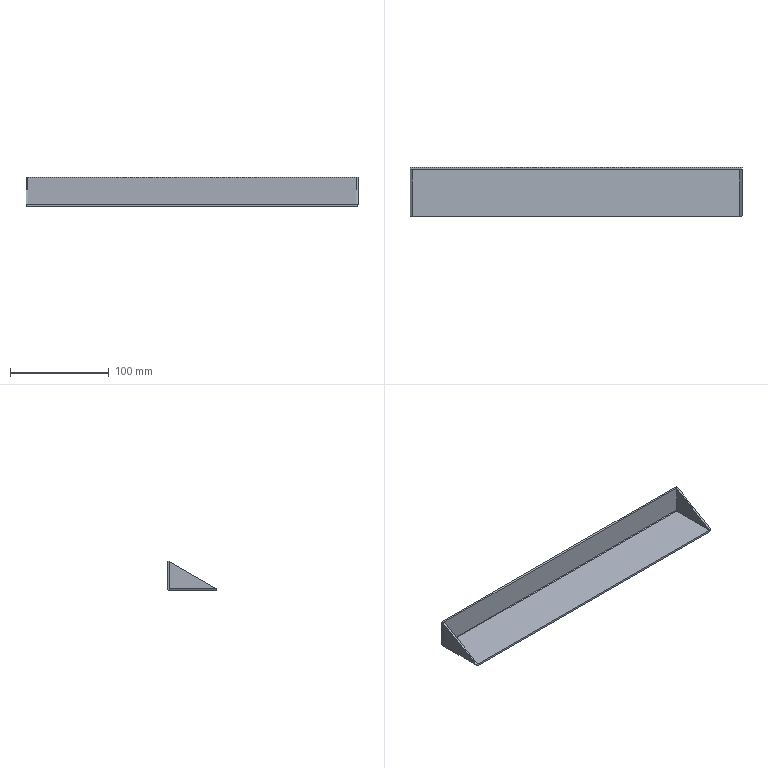Part | SolidWorks | features BaseBody 1 | 1 solid | 30 faces | box 336 x 50 x 30 mm | volume 54447 mm3 | plane 22 | cylinder 6 | spline 2 | commonest cylinder face diameters 1 x3 5 x3
STEP:
#1=CARTESIAN_POINT('',(166.,-24.136,0.5));
#2=VERTEX_POINT('',#1);
#3=CARTESIAN_POINT('',(166.,22.5,0.5));
#4=VERTEX_POINT('',#3);
#5=CARTESIAN_POINT('',(166.,-24.136,0.5));
#6=DIRECTION('',(0.,1.,0.));
#7=VECTOR('',#6,1000.);
#8=LINE('',#5,#7);
#9=EDGE_CURVE('',#2,#4,#8,.T.);
#10=ORIENTED_EDGE('',*,*,#9,.F.);
#11=CARTESIAN_POINT('',(166.,22.5,27.5));
#12=VERTEX_POINT('',#11);
#13=CARTESIAN_POINT('',(166.,22.5,27.5));
#14=DIRECTION('',(0.,-0.8654,-0.501));
#15=VECTOR('',#14,1000.);
#16=LINE('',#13,#15);
#17=EDGE_CURVE('',#12,#2,#16,.T.);
#18=ORIENTED_EDGE('',*,*,#17,.F.);
#19=CARTESIAN_POINT('',(166.,22.5,27.5));
#20=DIRECTION('',(0.,0.,1.));
#21=VECTOR('',#20,1000.);
#22=LINE('',#19,#21);
#23=EDGE_CURVE('',#4,#12,#22,.T.);
#24=ORIENTED_EDGE('',*,*,#23,.F.);
#25=EDGE_LOOP('',(#10,#18,#24));
#26=FACE_OUTER_BOUND('',#25,.T.);
#27=CARTESIAN_POINT('',(166.,0.,0.));
#28=DIRECTION('',(1.,0.,0.));
#29=DIRECTION('',(0.,0.,-1.));
#30=AXIS2_PLACEMENT_3D('',#27,#28,#29);
#31=PLANE('',#30);
#32=ADVANCED_FACE('',(#26),#31,.F.);
#33=CARTESIAN_POINT('',(168.,22.5,27.5));
#34=VERTEX_POINT('',#33);
#35=CARTESIAN_POINT('',(168.,-24.136,0.5));
#36=VERTEX_POINT('',#35);
#37=CARTESIAN_POINT('',(168.,-6.276,10.84));
#38=DIRECTION('',(0.,-0.8654,-0.501));
#39=VECTOR('',#38,1000.);
#40=LINE('',#37,#39);
#41=EDGE_CURVE('',#34,#36,#40,.T.);
#42=ORIENTED_EDGE('',*,*,#41,.T.);
#43=CARTESIAN_POINT('',(168.,22.5,0.5));
#44=VERTEX_POINT('',#43);
#45=CARTESIAN_POINT('',(168.,0.,0.5));
#46=DIRECTION('',(0.,1.,0.));
#47=VECTOR('',#46,1000.);
#48=LINE('',#45,#47);
#49=EDGE_CURVE('',#36,#44,#48,.T.);
#50=ORIENTED_EDGE('',*,*,#49,.T.);
#51=CARTESIAN_POINT('',(168.,22.5,0.));
#52=DIRECTION('',(0.,0.,1.));
#53=VECTOR('',#52,1000.);
#54=LINE('',#51,#53);
#55=EDGE_CURVE('',#44,#34,#54,.T.);
#56=ORIENTED_EDGE('',*,*,#55,.T.);
#57=EDGE_LOOP('',(#42,#50,#56));
#58=FACE_OUTER_BOUND('',#57,.T.);
#59=CARTESIAN_POINT('',(168.,0.,0.));
#60=DIRECTION('',(1.,0.,0.));
#61=DIRECTION('',(0.,0.,-1.));
#62=AXIS2_PLACEMENT_3D('',#59,#60,#61);
#63=PLANE('',#62);
#64=ADVANCED_FACE('',(#58),#63,.T.);
#65=CARTESIAN_POINT('',(166.,22.5,0.5));
#66=DIRECTION('',(1.,0.,0.));
#67=VECTOR('',#66,1000.);
#68=LINE('',#65,#67);
#69=EDGE_CURVE('',#4,#44,#68,.T.);
#70=ORIENTED_EDGE('',*,*,#69,.F.);
#71=ORIENTED_EDGE('',*,*,#23,.T.);
#72=CARTESIAN_POINT('',(168.,22.5,27.5));
#73=DIRECTION('',(-1.,0.,0.));
#74=VECTOR('',#73,1000.);
#75=LINE('',#72,#74);
#76=EDGE_CURVE('',#34,#12,#75,.T.);
#77=ORIENTED_EDGE('',*,*,#76,.F.);
#78=ORIENTED_EDGE('',*,*,#55,.F.);
#79=EDGE_LOOP('',(#70,#71,#77,#78));
#80=FACE_OUTER_BOUND('',#79,.T.);
#81=CARTESIAN_POINT('',(168.,22.5,27.5));
#82=DIRECTION('',(0.,-1.,0.));
#83=DIRECTION('',(-1.,0.,0.));
#84=AXIS2_PLACEMENT_3D('',#81,#82,#83);
#85=PLANE('',#84);
#86=ADVANCED_FACE('',(#80),#85,.F.);
#87=CARTESIAN_POINT('',(168.,-24.136,0.5));
#88=DIRECTION('',(1.,0.,0.));
#89=VECTOR('',#88,1000.);
#90=LINE('',#87,#89);
#91=EDGE_CURVE('',#2,#36,#90,.T.);
#92=ORIENTED_EDGE('',*,*,#91,.T.);
#93=ORIENTED_EDGE('',*,*,#41,.F.);
#94=ORIENTED_EDGE('',*,*,#76,.T.);
#95=ORIENTED_EDGE('',*,*,#17,.T.);
#96=EDGE_LOOP('',(#92,#93,#94,#95));
#97=FACE_OUTER_BOUND('',#96,.T.);
#98=CARTESIAN_POINT('',(168.,22.5,27.5));
#99=DIRECTION('',(0.,0.501,-0.8654));
#100=DIRECTION('',(-1.,0.,0.));
#101=AXIS2_PLACEMENT_3D('',#98,#99,#100);
#102=PLANE('',#101);
#103=ADVANCED_FACE('',(#97),#102,.F.);
#104=CARTESIAN_POINT('',(165.5,22.5,0.));
#105=VERTEX_POINT('',#104);
#106=CARTESIAN_POINT('',(165.5,-25.,0.));
#107=VERTEX_POINT('',#106);
#108=CARTESIAN_POINT('',(165.5,22.5,0.));
#109=DIRECTION('',(0.,-1.,0.));
#110=VECTOR('',#109,1000.);
#111=LINE('',#108,#110);
#112=EDGE_CURVE('',#105,#107,#111,.T.);
#113=ORIENTED_EDGE('',*,*,#112,.T.);
#114=CARTESIAN_POINT('',(165.5,-25.,0.));
#115=CARTESIAN_POINT('',(165.631,-24.856,0.));
#116=CARTESIAN_POINT('',(165.761,-24.712,0.05389));
#117=CARTESIAN_POINT('',(165.946,-24.424,0.239));
#118=CARTESIAN_POINT('',(166.,-24.28,0.3691));
#119=CARTESIAN_POINT('',(166.,-24.136,0.5));
#120=B_SPLINE_CURVE_WITH_KNOTS('',3,(#114,#115,#116,#117,#118,#119),.UNSPECIFIED.,.F.,.F.,(4,2,4),(0.,0.5,1.),.UNSPECIFIED.);
#121=EDGE_CURVE('',#107,#2,#120,.T.);
#122=ORIENTED_EDGE('',*,*,#121,.T.);
#123=ORIENTED_EDGE('',*,*,#9,.T.);
#124=CARTESIAN_POINT('',(165.5,22.5,0.5));
#125=DIRECTION('',(0.,1.,0.));
#126=DIRECTION('',(0.,0.,1.));
#127=AXIS2_PLACEMENT_3D('',#124,#125,#126);
#128=CIRCLE('',#127,0.5);
#129=EDGE_CURVE('',#4,#105,#128,.T.);
#130=ORIENTED_EDGE('',*,*,#129,.T.);
#131=EDGE_LOOP('',(#113,#122,#123,#130));
#132=FACE_OUTER_BOUND('',#131,.T.);
#133=CARTESIAN_POINT('',(165.5,22.5,0.5));
#134=DIRECTION('',(0.,1.,0.));
#135=DIRECTION('',(1.,0.,0.));
#136=AXIS2_PLACEMENT_3D('',#133,#134,#135);
#137=CYLINDRICAL_SURFACE('',#136,0.5);
#138=ADVANCED_FACE('',(#132),#137,.F.);
#139=CARTESIAN_POINT('',(165.5,22.5,-2.));
#140=VERTEX_POINT('',#139);
#141=CARTESIAN_POINT('',(165.5,-25.,-2.));
#142=VERTEX_POINT('',#141);
#143=CARTESIAN_POINT('',(165.5,22.5,-2.));
#144=DIRECTION('',(0.,-1.,0.));
#145=VECTOR('',#144,1000.);
#146=LINE('',#143,#145);
#147=EDGE_CURVE('',#140,#142,#146,.T.);
#148=ORIENTED_EDGE('',*,*,#147,.F.);
#149=CARTESIAN_POINT('',(165.5,22.5,0.5));
#150=DIRECTION('',(0.,1.,0.));
#151=DIRECTION('',(0.,0.,1.));
#152=AXIS2_PLACEMENT_3D('',#149,#150,#151);
#153=CIRCLE('',#152,2.5);
#154=EDGE_CURVE('',#44,#140,#153,.T.);
#155=ORIENTED_EDGE('',*,*,#154,.F.);
#156=ORIENTED_EDGE('',*,*,#49,.F.);
#157=CARTESIAN_POINT('',(165.5,-25.,-2.));
#158=CARTESIAN_POINT('',(165.827,-24.928,-2.));
#159=CARTESIAN_POINT('',(166.154,-24.856,-1.935));
#160=CARTESIAN_POINT('',(166.759,-24.712,-1.684));
#161=CARTESIAN_POINT('',(167.036,-24.64,-1.499));
#162=CARTESIAN_POINT('',(167.499,-24.496,-1.036));
#163=CARTESIAN_POINT('',(167.684,-24.424,-0.759));
#164=CARTESIAN_POINT('',(167.935,-24.28,-0.1544));
#165=CARTESIAN_POINT('',(168.,-24.208,0.1727));
#166=CARTESIAN_POINT('',(168.,-24.136,0.5));
#167=B_SPLINE_CURVE_WITH_KNOTS('',3,(#157,#158,#159,#160,#161,#162,#163,#164,#165,#166),.UNSPECIFIED.,.F.,.F.,(4,2,2,2,4),(0.,0.25,0.5,0.75,1.),.UNSPECIFIED.);
#168=EDGE_CURVE('',#142,#36,#167,.T.);
#169=ORIENTED_EDGE('',*,*,#168,.F.);
#170=EDGE_LOOP('',(#148,#155,#156,#169));
#171=FACE_OUTER_BOUND('',#170,.T.);
#172=CARTESIAN_POINT('',(165.5,22.5,0.5));
#173=DIRECTION('',(0.,1.,0.));
#174=DIRECTION('',(1.,0.,0.));
#175=AXIS2_PLACEMENT_3D('',#172,#173,#174);
#176=CYLINDRICAL_SURFACE('',#175,2.5);
#177=ADVANCED_FACE('',(#171),#176,.T.);
#178=ORIENTED_EDGE('',*,*,#129,.F.);
#179=ORIENTED_EDGE('',*,*,#69,.T.);
#180=ORIENTED_EDGE('',*,*,#154,.T.);
#181=CARTESIAN_POINT('',(165.5,22.5,0.));
#182=DIRECTION('',(0.,0.,-1.));
#183=VECTOR('',#182,1000.);
#184=LINE('',#181,#183);
#185=EDGE_CURVE('',#105,#140,#184,.T.);
#186=ORIENTED_EDGE('',*,*,#185,.F.);
#187=EDGE_LOOP('',(#178,#179,#180,#186));
#188=FACE_OUTER_BOUND('',#187,.T.);
#189=CARTESIAN_POINT('',(165.5,22.5,0.5));
#190=DIRECTION('',(0.,-1.,0.));
#191=DIRECTION('',(0.,0.,-1.));
#192=AXIS2_PLACEMENT_3D('',#189,#190,#191);
#193=PLANE('',#192);
#194=ADVANCED_FACE('',(#188),#193,.F.);
#195=ORIENTED_EDGE('',*,*,#91,.F.);
#196=ORIENTED_EDGE('',*,*,#121,.F.);
#197=CARTESIAN_POINT('',(165.5,-25.,0.));
#198=DIRECTION('',(0.,0.,-1.));
#199=VECTOR('',#198,1000.);
#200=LINE('',#197,#199);
#201=EDGE_CURVE('',#107,#142,#200,.T.);
#202=ORIENTED_EDGE('',*,*,#201,.T.);
#203=ORIENTED_EDGE('',*,*,#168,.T.);
#204=EDGE_LOOP('',(#195,#196,#202,#203));
#205=FACE_OUTER_BOUND('',#204,.T.);
#206=CARTESIAN_POINT('',(165.5,-25.,-2.02));
#207=CARTESIAN_POINT('',(165.83,-24.928,-2.02));
#208=CARTESIAN_POINT('',(166.16,-24.856,-1.954));
#209=CARTESIAN_POINT('',(166.769,-24.712,-1.702));
#210=CARTESIAN_POINT('',(167.049,-24.64,-1.515));
#211=CARTESIAN_POINT('',(167.515,-24.496,-1.049));
#212=CARTESIAN_POINT('',(167.702,-24.424,-0.7691));
#213=CARTESIAN_POINT('',(167.954,-24.28,-0.1596));
#214=CARTESIAN_POINT('',(168.02,-24.208,0.1701));
#215=CARTESIAN_POINT('',(168.02,-24.136,0.5));
#216=CARTESIAN_POINT('',(165.5,-25.,-2.));
#217=CARTESIAN_POINT('',(165.827,-24.928,-2.));
#218=CARTESIAN_POINT('',(166.154,-24.856,-1.935));
#219=CARTESIAN_POINT('',(166.759,-24.712,-1.684));
#220=CARTESIAN_POINT('',(167.036,-24.64,-1.499));
#221=CARTESIAN_POINT('',(167.499,-24.496,-1.036));
#222=CARTESIAN_POINT('',(167.684,-24.424,-0.759));
#223=CARTESIAN_POINT('',(167.935,-24.28,-0.1544));
#224=CARTESIAN_POINT('',(168.,-24.208,0.1727));
#225=CARTESIAN_POINT('',(168.,-24.136,0.5));
#226=CARTESIAN_POINT('',(165.5,-25.,0.));
#227=CARTESIAN_POINT('',(165.565,-24.928,0.));
#228=CARTESIAN_POINT('',(165.631,-24.856,0.01301));
#229=CARTESIAN_POINT('',(165.752,-24.712,0.06311));
#230=CARTESIAN_POINT('',(165.807,-24.64,0.1002));
#231=CARTESIAN_POINT('',(165.9,-24.496,0.1927));
#232=CARTESIAN_POINT('',(165.937,-24.424,0.2482));
#233=CARTESIAN_POINT('',(165.987,-24.28,0.3691));
#234=CARTESIAN_POINT('',(166.,-24.208,0.4345));
#235=CARTESIAN_POINT('',(166.,-24.136,0.5));
#236=CARTESIAN_POINT('',(165.5,-25.,0.0202));
#237=CARTESIAN_POINT('',(165.563,-24.928,0.0202));
#238=CARTESIAN_POINT('',(165.626,-24.856,0.03269));
#239=CARTESIAN_POINT('',(165.742,-24.712,0.08076));
#240=CARTESIAN_POINT('',(165.795,-24.64,0.1163));
#241=CARTESIAN_POINT('',(165.884,-24.496,0.2051));
#242=CARTESIAN_POINT('',(165.919,-24.424,0.2584));
#243=CARTESIAN_POINT('',(165.967,-24.28,0.3744));
#244=CARTESIAN_POINT('',(165.98,-24.208,0.4372));
#245=CARTESIAN_POINT('',(165.98,-24.136,0.5));
#246=B_SPLINE_SURFACE_WITH_KNOTS('',1,3,((#206,#207,#208,#209,#210,#211,#212,#213,#214,#215),(#216,#217,#218,#219,#220,#221,#222,#223,#224,#225),(#226,#227,#228,#229,#230,#231,#232,#233,#234,#235),(#236,#237,#238,#239,#240,#241,#242,#243,#244,#245)),.UNSPECIFIED.,.F.,.F.,.F.,(2,1,1,2),(4,2,2,2,4),(-0.01,0.,1.,1.01),(0.,0.25,0.5,0.75,1.),.UNSPECIFIED.);
#247=ADVANCED_FACE('',(#205),#246,.F.);
#248=CARTESIAN_POINT('',(-166.,-24.136,0.5));
#249=VERTEX_POINT('',#248);
#250=CARTESIAN_POINT('',(-166.,22.5,27.5));
#251=VERTEX_POINT('',#250);
#252=CARTESIAN_POINT('',(-166.,22.5,27.5));
#253=DIRECTION('',(0.,0.8654,0.501));
#254=VECTOR('',#253,1000.);
#255=LINE('',#252,#254);
#256=EDGE_CURVE('',#249,#251,#255,.T.);
#257=ORIENTED_EDGE('',*,*,#256,.F.);
#258=CARTESIAN_POINT('',(-166.,22.5,0.5));
#259=VERTEX_POINT('',#258);
#260=CARTESIAN_POINT('',(-166.,22.5,0.5));
#261=DIRECTION('',(0.,-1.,0.));
#262=VECTOR('',#261,1000.);
#263=LINE('',#260,#262);
#264=EDGE_CURVE('',#259,#249,#263,.T.);
#265=ORIENTED_EDGE('',*,*,#264,.F.);
#266=CARTESIAN_POINT('',(-166.,22.5,0.));
#267=DIRECTION('',(0.,0.,-1.));
#268=VECTOR('',#267,1000.);
#269=LINE('',#266,#268);
#270=EDGE_CURVE('',#251,#259,#269,.T.);
#271=ORIENTED_EDGE('',*,*,#270,.F.);
#272=EDGE_LOOP('',(#257,#265,#271));
#273=FACE_OUTER_BOUND('',#272,.T.);
#274=CARTESIAN_POINT('',(-166.,0.,0.));
#275=DIRECTION('',(1.,0.,0.));
#276=DIRECTION('',(0.,0.,1.));
#277=AXIS2_PLACEMENT_3D('',#274,#275,#276);
#278=PLANE('',#277);
#279=ADVANCED_FACE('',(#273),#278,.T.);
#280=CARTESIAN_POINT('',(-168.,-24.136,0.5));
#281=VERTEX_POINT('',#280);
#282=CARTESIAN_POINT('',(-168.,22.5,0.5));
#283=VERTEX_POINT('',#282);
#284=CARTESIAN_POINT('',(-168.,22.5,0.5));
#285=DIRECTION('',(0.,1.,0.));
#286=VECTOR('',#285,1000.);
#287=LINE('',#284,#286);
#288=EDGE_CURVE('',#281,#283,#287,.T.);
#289=ORIENTED_EDGE('',*,*,#288,.F.);
#290=CARTESIAN_POINT('',(-168.,22.5,27.5));
#291=VERTEX_POINT('',#290);
#292=CARTESIAN_POINT('',(-168.,-6.276,10.84));
#293=DIRECTION('',(0.,0.8654,0.501));
#294=VECTOR('',#293,1000.);
#295=LINE('',#292,#294);
#296=EDGE_CURVE('',#281,#291,#295,.T.);
#297=ORIENTED_EDGE('',*,*,#296,.T.);
#298=CARTESIAN_POINT('',(-168.,22.5,0.));
#299=DIRECTION('',(0.,0.,-1.));
#300=VECTOR('',#299,1000.);
#301=LINE('',#298,#300);
#302=EDGE_CURVE('',#291,#283,#301,.T.);
#303=ORIENTED_EDGE('',*,*,#302,.T.);
#304=EDGE_LOOP('',(#289,#297,#303));
#305=FACE_OUTER_BOUND('',#304,.T.);
#306=CARTESIAN_POINT('',(-168.,0.,0.));
#307=DIRECTION('',(1.,0.,0.));
#308=DIRECTION('',(0.,0.,1.));
#309=AXIS2_PLACEMENT_3D('',#306,#307,#308);
#310=PLANE('',#309);
#311=ADVANCED_FACE('',(#305),#310,.F.);
#312=CARTESIAN_POINT('',(-166.,-24.136,0.5));
#313=DIRECTION('',(-1.,0.,0.));
#314=VECTOR('',#313,1000.);
#315=LINE('',#312,#314);
#316=EDGE_CURVE('',#249,#281,#315,.T.);
#317=ORIENTED_EDGE('',*,*,#316,.F.);
#318=ORIENTED_EDGE('',*,*,#256,.T.);
#319=CARTESIAN_POINT('',(-168.,22.5,27.5));
#320=DIRECTION('',(1.,0.,0.));
#321=VECTOR('',#320,1000.);
#322=LINE('',#319,#321);
#323=EDGE_CURVE('',#291,#251,#322,.T.);
#324=ORIENTED_EDGE('',*,*,#323,.F.);
#325=ORIENTED_EDGE('',*,*,#296,.F.);
#326=EDGE_LOOP('',(#317,#318,#324,#325));
#327=FACE_OUTER_BOUND('',#326,.T.);
#328=CARTESIAN_POINT('',(-168.,22.5,27.5));
#329=DIRECTION('',(0.,0.501,-0.8654));
#330=DIRECTION('',(-1.,0.,0.));
#331=AXIS2_PLACEMENT_3D('',#328,#329,#330);
#332=PLANE('',#331);
#333=ADVANCED_FACE('',(#327),#332,.F.);
#334=CARTESIAN_POINT('',(-168.,22.5,0.5));
#335=DIRECTION('',(-1.,0.,0.));
#336=VECTOR('',#335,1000.);
#337=LINE('',#334,#336);
#338=EDGE_CURVE('',#259,#283,#337,.T.);
#339=ORIENTED_EDGE('',*,*,#338,.T.);
#340=ORIENTED_EDGE('',*,*,#302,.F.);
#341=ORIENTED_EDGE('',*,*,#323,.T.);
#342=ORIENTED_EDGE('',*,*,#270,.T.);
#343=EDGE_LOOP('',(#339,#340,#341,#342));
#344=FACE_OUTER_BOUND('',#343,.T.);
#345=CARTESIAN_POINT('',(-168.,22.5,0.));
#346=DIRECTION('',(0.,-1.,0.));
#347=DIRECTION('',(-1.,0.,0.));
#348=AXIS2_PLACEMENT_3D('',#345,#346,#347);
#349=PLANE('',#348);
#350=ADVANCED_FACE('',(#344),#349,.F.);
#351=CARTESIAN_POINT('',(-165.5,-25.,0.));
#352=VERTEX_POINT('',#351);
#353=CARTESIAN_POINT('',(-165.5,22.5,0.));
#354=VERTEX_POINT('',#353);
#355=CARTESIAN_POINT('',(-165.5,-25.,0.));
#356=DIRECTION('',(0.,1.,0.));
#357=VECTOR('',#356,1000.);
#358=LINE('',#355,#357);
#359=EDGE_CURVE('',#352,#354,#358,.T.);
#360=ORIENTED_EDGE('',*,*,#359,.T.);
#361=CARTESIAN_POINT('',(-165.5,22.5,0.5));
#362=DIRECTION('',(0.,1.,0.));
#363=DIRECTION('',(0.,0.,-1.));
#364=AXIS2_PLACEMENT_3D('',#361,#362,#363);
#365=CIRCLE('',#364,0.5);
#366=EDGE_CURVE('',#354,#259,#365,.T.);
#367=ORIENTED_EDGE('',*,*,#366,.T.);
#368=ORIENTED_EDGE('',*,*,#264,.T.);
#369=CARTESIAN_POINT('',(-166.,-24.136,0.5));
#370=CARTESIAN_POINT('',(-166.,-24.28,0.3691));
#371=CARTESIAN_POINT('',(-165.946,-24.424,0.239));
#372=CARTESIAN_POINT('',(-165.761,-24.712,0.05389));
#373=CARTESIAN_POINT('',(-165.631,-24.856,0.));
#374=CARTESIAN_POINT('',(-165.5,-25.,0.));
#375=B_SPLINE_CURVE_WITH_KNOTS('',3,(#369,#370,#371,#372,#373,#374),.UNSPECIFIED.,.F.,.F.,(4,2,4),(0.,0.5,1.),.UNSPECIFIED.);
#376=EDGE_CURVE('',#249,#352,#375,.T.);
#377=ORIENTED_EDGE('',*,*,#376,.T.);
#378=EDGE_LOOP('',(#360,#367,#368,#377));
#379=FACE_OUTER_BOUND('',#378,.T.);
#380=CARTESIAN_POINT('',(-165.5,-25.,0.5));
#381=DIRECTION('',(0.,-1.,0.));
#382=DIRECTION('',(-1.,0.,0.));
#383=AXIS2_PLACEMENT_3D('',#380,#381,#382);
#384=CYLINDRICAL_SURFACE('',#383,0.5);
#385=ADVANCED_FACE('',(#379),#384,.F.);
#386=CARTESIAN_POINT('',(-165.5,-25.,-2.));
#387=VERTEX_POINT('',#386);
#388=CARTESIAN_POINT('',(-165.5,22.5,-2.));
#389=VERTEX_POINT('',#388);
#390=CARTESIAN_POINT('',(-165.5,-25.,-2.));
#391=DIRECTION('',(0.,1.,0.));
#392=VECTOR('',#391,1000.);
#393=LINE('',#390,#392);
#394=EDGE_CURVE('',#387,#389,#393,.T.);
#395=ORIENTED_EDGE('',*,*,#394,.F.);
#396=CARTESIAN_POINT('',(-168.,-24.136,0.5));
#397=CARTESIAN_POINT('',(-168.,-24.208,0.1727));
#398=CARTESIAN_POINT('',(-167.935,-24.28,-0.1544));
#399=CARTESIAN_POINT('',(-167.684,-24.424,-0.759));
#400=CARTESIAN_POINT('',(-167.499,-24.496,-1.036));
#401=CARTESIAN_POINT('',(-167.036,-24.64,-1.499));
#402=CARTESIAN_POINT('',(-166.759,-24.712,-1.684));
#403=CARTESIAN_POINT('',(-166.154,-24.856,-1.935));
#404=CARTESIAN_POINT('',(-165.827,-24.928,-2.));
#405=CARTESIAN_POINT('',(-165.5,-25.,-2.));
#406=B_SPLINE_CURVE_WITH_KNOTS('',3,(#396,#397,#398,#399,#400,#401,#402,#403,#404,#405),.UNSPECIFIED.,.F.,.F.,(4,2,2,2,4),(0.,0.25,0.5,0.75,1.),.UNSPECIFIED.);
#407=EDGE_CURVE('',#281,#387,#406,.T.);
#408=ORIENTED_EDGE('',*,*,#407,.F.);
#409=ORIENTED_EDGE('',*,*,#288,.T.);
#410=CARTESIAN_POINT('',(-165.5,22.5,0.5));
#411=DIRECTION('',(0.,1.,0.));
#412=DIRECTION('',(0.,0.,-1.));
#413=AXIS2_PLACEMENT_3D('',#410,#411,#412);
#414=CIRCLE('',#413,2.5);
#415=EDGE_CURVE('',#389,#283,#414,.T.);
#416=ORIENTED_EDGE('',*,*,#415,.F.);
#417=EDGE_LOOP('',(#395,#408,#409,#416));
#418=FACE_OUTER_BOUND('',#417,.T.);
#419=CARTESIAN_POINT('',(-165.5,-25.,0.5));
#420=DIRECTION('',(0.,-1.,0.));
#421=DIRECTION('',(-1.,0.,0.));
#422=AXIS2_PLACEMENT_3D('',#419,#420,#421);
#423=CYLINDRICAL_SURFACE('',#422,2.5);
#424=ADVANCED_FACE('',(#418),#423,.T.);
#425=ORIENTED_EDGE('',*,*,#376,.F.);
#426=ORIENTED_EDGE('',*,*,#316,.T.);
#427=ORIENTED_EDGE('',*,*,#407,.T.);
#428=CARTESIAN_POINT('',(-165.5,-25.,0.));
#429=DIRECTION('',(0.,0.,-1.));
#430=VECTOR('',#429,1000.);
#431=LINE('',#428,#430);
#432=EDGE_CURVE('',#352,#387,#431,.T.);
#433=ORIENTED_EDGE('',*,*,#432,.F.);
#434=EDGE_LOOP('',(#425,#426,#427,#433));
#435=FACE_OUTER_BOUND('',#434,.T.);
#436=CARTESIAN_POINT('',(-168.02,-24.136,0.5));
#437=CARTESIAN_POINT('',(-168.02,-24.208,0.1701));
#438=CARTESIAN_POINT('',(-167.954,-24.28,-0.1596));
#439=CARTESIAN_POINT('',(-167.702,-24.424,-0.7691));
#440=CARTESIAN_POINT('',(-167.515,-24.496,-1.049));
#441=CARTESIAN_POINT('',(-167.049,-24.64,-1.515));
#442=CARTESIAN_POINT('',(-166.769,-24.712,-1.702));
#443=CARTESIAN_POINT('',(-166.16,-24.856,-1.954));
#444=CARTESIAN_POINT('',(-165.83,-24.928,-2.02));
#445=CARTESIAN_POINT('',(-165.5,-25.,-2.02));
#446=CARTESIAN_POINT('',(-168.,-24.136,0.5));
#447=CARTESIAN_POINT('',(-168.,-24.208,0.1727));
#448=CARTESIAN_POINT('',(-167.935,-24.28,-0.1544));
#449=CARTESIAN_POINT('',(-167.684,-24.424,-0.759));
#450=CARTESIAN_POINT('',(-167.499,-24.496,-1.036));
#451=CARTESIAN_POINT('',(-167.036,-24.64,-1.499));
#452=CARTESIAN_POINT('',(-166.759,-24.712,-1.684));
#453=CARTESIAN_POINT('',(-166.154,-24.856,-1.935));
#454=CARTESIAN_POINT('',(-165.827,-24.928,-2.));
#455=CARTESIAN_POINT('',(-165.5,-25.,-2.));
#456=CARTESIAN_POINT('',(-166.,-24.136,0.5));
#457=CARTESIAN_POINT('',(-166.,-24.208,0.4345));
#458=CARTESIAN_POINT('',(-165.987,-24.28,0.3691));
#459=CARTESIAN_POINT('',(-165.937,-24.424,0.2482));
#460=CARTESIAN_POINT('',(-165.9,-24.496,0.1927));
#461=CARTESIAN_POINT('',(-165.807,-24.64,0.1002));
#462=CARTESIAN_POINT('',(-165.752,-24.712,0.06311));
#463=CARTESIAN_POINT('',(-165.631,-24.856,0.01301));
#464=CARTESIAN_POINT('',(-165.565,-24.928,0.));
#465=CARTESIAN_POINT('',(-165.5,-25.,0.));
#466=CARTESIAN_POINT('',(-165.98,-24.136,0.5));
#467=CARTESIAN_POINT('',(-165.98,-24.208,0.4372));
#468=CARTESIAN_POINT('',(-165.967,-24.28,0.3744));
#469=CARTESIAN_POINT('',(-165.919,-24.424,0.2584));
#470=CARTESIAN_POINT('',(-165.884,-24.496,0.2051));
#471=CARTESIAN_POINT('',(-165.795,-24.64,0.1163));
#472=CARTESIAN_POINT('',(-165.742,-24.712,0.08076));
#473=CARTESIAN_POINT('',(-165.626,-24.856,0.03269));
#474=CARTESIAN_POINT('',(-165.563,-24.928,0.0202));
#475=CARTESIAN_POINT('',(-165.5,-25.,0.0202));
#476=B_SPLINE_SURFACE_WITH_KNOTS('',1,3,((#436,#437,#438,#439,#440,#441,#442,#443,#444,#445),(#446,#447,#448,#449,#450,#451,#452,#453,#454,#455),(#456,#457,#458,#459,#460,#461,#462,#463,#464,#465),(#466,#467,#468,#469,#470,#471,#472,#473,#474,#475)),.UNSPECIFIED.,.F.,.F.,.F.,(2,1,1,2),(4,2,2,2,4),(-0.01,0.,1.,1.01),(0.,0.25,0.5,0.75,1.),.UNSPECIFIED.);
#477=ADVANCED_FACE('',(#435),#476,.F.);
#478=ORIENTED_EDGE('',*,*,#338,.F.);
#479=ORIENTED_EDGE('',*,*,#366,.F.);
#480=CARTESIAN_POINT('',(-165.5,22.5,0.));
#481=DIRECTION('',(0.,0.,-1.));
#482=VECTOR('',#481,1000.);
#483=LINE('',#480,#482);
#484=EDGE_CURVE('',#354,#389,#483,.T.);
#485=ORIENTED_EDGE('',*,*,#484,.T.);
#486=ORIENTED_EDGE('',*,*,#415,.T.);
#487=EDGE_LOOP('',(#478,#479,#485,#486));
#488=FACE_OUTER_BOUND('',#487,.T.);
#489=CARTESIAN_POINT('',(-165.5,22.5,0.5));
#490=DIRECTION('',(0.,1.,0.));
#491=DIRECTION('',(0.,0.,-1.));
#492=AXIS2_PLACEMENT_3D('',#489,#490,#491);
#493=PLANE('',#492);
#494=ADVANCED_FACE('',(#488),#493,.T.);
#495=CARTESIAN_POINT('',(-168.,23.,28.));
#496=VERTEX_POINT('',#495);
#497=CARTESIAN_POINT('',(168.,23.,28.));
#498=VERTEX_POINT('',#497);
#499=CARTESIAN_POINT('',(168.,23.,28.));
#500=DIRECTION('',(1.,0.,0.));
#501=VECTOR('',#500,1000.);
#502=LINE('',#499,#501);
#503=EDGE_CURVE('',#496,#498,#502,.T.);
#504=ORIENTED_EDGE('',*,*,#503,.T.);
#505=CARTESIAN_POINT('',(168.,25.,28.));
#506=VERTEX_POINT('',#505);
#507=CARTESIAN_POINT('',(168.,25.,28.));
#508=DIRECTION('',(0.,-1.,0.));
#509=VECTOR('',#508,1000.);
#510=LINE('',#507,#509);
#511=EDGE_CURVE('',#506,#498,#510,.T.);
#512=ORIENTED_EDGE('',*,*,#511,.F.);
#513=CARTESIAN_POINT('',(-168.,25.,28.));
#514=VERTEX_POINT('',#513);
#515=CARTESIAN_POINT('',(0.,25.,28.));
#516=DIRECTION('',(1.,0.,0.));
#517=VECTOR('',#516,1000.);
#518=LINE('',#515,#517);
#519=EDGE_CURVE('',#514,#506,#518,.T.);
#520=ORIENTED_EDGE('',*,*,#519,.F.);
#521=CARTESIAN_POINT('',(-168.,25.,28.));
#522=DIRECTION('',(0.,-1.,0.));
#523=VECTOR('',#522,1000.);
#524=LINE('',#521,#523);
#525=EDGE_CURVE('',#514,#496,#524,.T.);
#526=ORIENTED_EDGE('',*,*,#525,.T.);
#527=EDGE_LOOP('',(#504,#512,#520,#526));
#528=FACE_OUTER_BOUND('',#527,.T.);
#529=CARTESIAN_POINT('',(168.,25.,28.));
#530=DIRECTION('',(0.,0.,-1.));
#531=DIRECTION('',(0.,-1.,0.));
#532=AXIS2_PLACEMENT_3D('',#529,#530,#531);
#533=PLANE('',#532);
#534=ADVANCED_FACE('',(#528),#533,.F.);
#535=CARTESIAN_POINT('',(-168.,23.,0.5));
#536=VERTEX_POINT('',#535);
#537=CARTESIAN_POINT('',(-168.,23.,28.));
#538=DIRECTION('',(0.,0.,1.));
#539=VECTOR('',#538,1000.);
#540=LINE('',#537,#539);
#541=EDGE_CURVE('',#536,#496,#540,.T.);
#542=ORIENTED_EDGE('',*,*,#541,.F.);
#543=CARTESIAN_POINT('',(-165.5,23.,0.5));
#544=VERTEX_POINT('',#543);
#545=CARTESIAN_POINT('',(168.,23.,0.5));
#546=DIRECTION('',(-1.,0.,0.));
#547=VECTOR('',#546,1000.);
#548=LINE('',#545,#547);
#549=EDGE_CURVE('',#544,#536,#548,.T.);
#550=ORIENTED_EDGE('',*,*,#549,.F.);
#551=CARTESIAN_POINT('',(165.5,23.,0.5));
#552=VERTEX_POINT('',#551);
#553=CARTESIAN_POINT('',(168.,23.,0.5));
#554=DIRECTION('',(-1.,0.,0.));
#555=VECTOR('',#554,1000.);
#556=LINE('',#553,#555);
#557=EDGE_CURVE('',#552,#544,#556,.T.);
#558=ORIENTED_EDGE('',*,*,#557,.F.);
#559=CARTESIAN_POINT('',(168.,23.,0.5));
#560=VERTEX_POINT('',#559);
#561=CARTESIAN_POINT('',(168.,23.,0.5));
#562=DIRECTION('',(-1.,0.,0.));
#563=VECTOR('',#562,1000.);
#564=LINE('',#561,#563);
#565=EDGE_CURVE('',#560,#552,#564,.T.);
#566=ORIENTED_EDGE('',*,*,#565,.F.);
#567=CARTESIAN_POINT('',(168.,23.,0.));
#568=DIRECTION('',(0.,0.,-1.));
#569=VECTOR('',#568,1000.);
#570=LINE('',#567,#569);
#571=EDGE_CURVE('',#498,#560,#570,.T.);
#572=ORIENTED_EDGE('',*,*,#571,.F.);
#573=ORIENTED_EDGE('',*,*,#503,.F.);
#574=EDGE_LOOP('',(#542,#550,#558,#566,#572,#573));
#575=FACE_OUTER_BOUND('',#574,.T.);
#576=CARTESIAN_POINT('',(0.,23.,0.));
#577=DIRECTION('',(0.,-1.,0.));
#578=DIRECTION('',(-1.,0.,0.));
#579=AXIS2_PLACEMENT_3D('',#576,#577,#578);
#580=PLANE('',#579);
#581=ADVANCED_FACE('',(#575),#580,.T.);
#582=CARTESIAN_POINT('',(-168.,25.,0.5));
#583=VERTEX_POINT('',#582);
#584=CARTESIAN_POINT('',(-165.5,25.,0.5));
#585=VERTEX_POINT('',#584);
#586=CARTESIAN_POINT('',(168.,25.,0.5));
#587=DIRECTION('',(1.,0.,0.));
#588=VECTOR('',#587,1000.);
#589=LINE('',#586,#588);
#590=EDGE_CURVE('',#583,#585,#589,.T.);
#591=ORIENTED_EDGE('',*,*,#590,.F.);
#592=CARTESIAN_POINT('',(-168.,25.,0.));
#593=DIRECTION('',(0.,0.,1.));
#594=VECTOR('',#593,1000.);
#595=LINE('',#592,#594);
#596=EDGE_CURVE('',#583,#514,#595,.T.);
#597=ORIENTED_EDGE('',*,*,#596,.T.);
#598=ORIENTED_EDGE('',*,*,#519,.T.);
#599=CARTESIAN_POINT('',(168.,25.,0.5));
#600=VERTEX_POINT('',#599);
#601=CARTESIAN_POINT('',(168.,25.,0.));
#602=DIRECTION('',(0.,0.,-1.));
#603=VECTOR('',#602,1000.);
#604=LINE('',#601,#603);
#605=EDGE_CURVE('',#506,#600,#604,.T.);
#606=ORIENTED_EDGE('',*,*,#605,.T.);
#607=CARTESIAN_POINT('',(165.5,25.,0.5));
#608=VERTEX_POINT('',#607);
#609=CARTESIAN_POINT('',(168.,25.,0.5));
#610=DIRECTION('',(1.,0.,0.));
#611=VECTOR('',#610,1000.);
#612=LINE('',#609,#611);
#613=EDGE_CURVE('',#608,#600,#612,.T.);
#614=ORIENTED_EDGE('',*,*,#613,.F.);
#615=CARTESIAN_POINT('',(168.,25.,0.5));
#616=DIRECTION('',(1.,0.,0.));
#617=VECTOR('',#616,1000.);
#618=LINE('',#615,#617);
#619=EDGE_CURVE('',#585,#608,#618,.T.);
#620=ORIENTED_EDGE('',*,*,#619,.F.);
#621=EDGE_LOOP('',(#591,#597,#598,#606,#614,#620));
#622=FACE_OUTER_BOUND('',#621,.T.);
#623=CARTESIAN_POINT('',(0.,25.,0.));
#624=DIRECTION('',(0.,-1.,0.));
#625=DIRECTION('',(-1.,0.,0.));
#626=AXIS2_PLACEMENT_3D('',#623,#624,#625);
#627=PLANE('',#626);
#628=ADVANCED_FACE('',(#622),#627,.F.);
#629=CARTESIAN_POINT('',(168.,25.,0.5));
#630=DIRECTION('',(0.,1.,0.));
#631=VECTOR('',#630,1000.);
#632=LINE('',#629,#631);
#633=EDGE_CURVE('',#560,#600,#632,.T.);
#634=ORIENTED_EDGE('',*,*,#633,.T.);
#635=ORIENTED_EDGE('',*,*,#605,.F.);
#636=ORIENTED_EDGE('',*,*,#511,.T.);
#637=ORIENTED_EDGE('',*,*,#571,.T.);
#638=EDGE_LOOP('',(#634,#635,#636,#637));
#639=FACE_OUTER_BOUND('',#638,.T.);
#640=CARTESIAN_POINT('',(168.,25.,0.));
#641=DIRECTION('',(-1.,0.,0.));
#642=DIRECTION('',(0.,1.,0.));
#643=AXIS2_PLACEMENT_3D('',#640,#641,#642);
#644=PLANE('',#643);
#645=ADVANCED_FACE('',(#639),#644,.F.);
#646=CARTESIAN_POINT('',(-168.,23.,0.5));
#647=DIRECTION('',(0.,1.,0.));
#648=VECTOR('',#647,1000.);
#649=LINE('',#646,#648);
#650=EDGE_CURVE('',#536,#583,#649,.T.);
#651=ORIENTED_EDGE('',*,*,#650,.F.);
#652=ORIENTED_EDGE('',*,*,#541,.T.);
#653=ORIENTED_EDGE('',*,*,#525,.F.);
#654=ORIENTED_EDGE('',*,*,#596,.F.);
#655=EDGE_LOOP('',(#651,#652,#653,#654));
#656=FACE_OUTER_BOUND('',#655,.T.);
#657=CARTESIAN_POINT('',(-168.,25.,28.));
#658=DIRECTION('',(1.,0.,0.));
#659=DIRECTION('',(0.,1.,0.));
#660=AXIS2_PLACEMENT_3D('',#657,#658,#659);
#661=PLANE('',#660);
#662=ADVANCED_FACE('',(#656),#661,.F.);
#663=CARTESIAN_POINT('',(165.5,22.5,0.5));
#664=DIRECTION('',(-1.,0.,0.));
#665=DIRECTION('',(0.,0.,-1.));
#666=AXIS2_PLACEMENT_3D('',#663,#664,#665);
#667=CIRCLE('',#666,0.5);
#668=EDGE_CURVE('',#552,#105,#667,.T.);
#669=ORIENTED_EDGE('',*,*,#668,.F.);
#670=ORIENTED_EDGE('',*,*,#557,.T.);
#671=CARTESIAN_POINT('',(-165.5,22.5,0.5));
#672=DIRECTION('',(1.,0.,0.));
#673=DIRECTION('',(0.,0.,1.));
#674=AXIS2_PLACEMENT_3D('',#671,#672,#673);
#675=CIRCLE('',#674,0.5);
#676=EDGE_CURVE('',#354,#544,#675,.T.);
#677=ORIENTED_EDGE('',*,*,#676,.F.);
#678=CARTESIAN_POINT('',(-168.,22.5,0.));
#679=DIRECTION('',(1.,0.,0.));
#680=VECTOR('',#679,1000.);
#681=LINE('',#678,#680);
#682=EDGE_CURVE('',#354,#105,#681,.T.);
#683=ORIENTED_EDGE('',*,*,#682,.T.);
#684=EDGE_LOOP('',(#669,#670,#677,#683));
#685=FACE_OUTER_BOUND('',#684,.T.);
#686=CARTESIAN_POINT('',(-168.,22.5,0.5));
#687=DIRECTION('',(-1.,0.,0.));
#688=DIRECTION('',(0.,1.,0.));
#689=AXIS2_PLACEMENT_3D('',#686,#687,#688);
#690=CYLINDRICAL_SURFACE('',#689,0.5);
#691=ADVANCED_FACE('',(#685),#690,.F.);
#692=ORIENTED_EDGE('',*,*,#201,.F.);
#693=CARTESIAN_POINT('',(168.,-25.,0.));
#694=DIRECTION('',(1.,0.,0.));
#695=VECTOR('',#694,1000.);
#696=LINE('',#693,#695);
#697=EDGE_CURVE('',#352,#107,#696,.T.);
#698=ORIENTED_EDGE('',*,*,#697,.F.);
#699=ORIENTED_EDGE('',*,*,#432,.T.);
#700=CARTESIAN_POINT('',(168.,-25.,-2.));
#701=DIRECTION('',(1.,0.,0.));
#702=VECTOR('',#701,1000.);
#703=LINE('',#700,#702);
#704=EDGE_CURVE('',#387,#142,#703,.T.);
#705=ORIENTED_EDGE('',*,*,#704,.T.);
#706=EDGE_LOOP('',(#692,#698,#699,#705));
#707=FACE_OUTER_BOUND('',#706,.T.);
#708=CARTESIAN_POINT('',(168.,-25.,-2.));
#709=DIRECTION('',(0.,-1.,0.));
#710=DIRECTION('',(0.,0.,-1.));
#711=AXIS2_PLACEMENT_3D('',#708,#709,#710);
#712=PLANE('',#711);
#713=ADVANCED_FACE('',(#707),#712,.T.);
#714=ORIENTED_EDGE('',*,*,#676,.T.);
#715=CARTESIAN_POINT('',(-165.5,23.,0.5));
#716=DIRECTION('',(0.,1.,0.));
#717=VECTOR('',#716,1000.);
#718=LINE('',#715,#717);
#719=EDGE_CURVE('',#544,#585,#718,.T.);
#720=ORIENTED_EDGE('',*,*,#719,.T.);
#721=CARTESIAN_POINT('',(-165.5,22.5,0.5));
#722=DIRECTION('',(1.,0.,0.));
#723=DIRECTION('',(0.,0.,1.));
#724=AXIS2_PLACEMENT_3D('',#721,#722,#723);
#725=CIRCLE('',#724,2.5);
#726=EDGE_CURVE('',#389,#585,#725,.T.);
#727=ORIENTED_EDGE('',*,*,#726,.F.);
#728=ORIENTED_EDGE('',*,*,#484,.F.);
#729=EDGE_LOOP('',(#714,#720,#727,#728));
#730=FACE_OUTER_BOUND('',#729,.T.);
#731=CARTESIAN_POINT('',(-165.5,22.5,0.5));
#732=DIRECTION('',(-1.,0.,0.));
#733=DIRECTION('',(0.,0.,1.));
#734=AXIS2_PLACEMENT_3D('',#731,#732,#733);
#735=PLANE('',#734);
#736=ADVANCED_FACE('',(#730),#735,.T.);
#737=CARTESIAN_POINT('',(165.5,22.5,0.5));
#738=DIRECTION('',(-1.,0.,0.));
#739=DIRECTION('',(0.,0.,-1.));
#740=AXIS2_PLACEMENT_3D('',#737,#738,#739);
#741=CIRCLE('',#740,2.5);
#742=EDGE_CURVE('',#608,#140,#741,.T.);
#743=ORIENTED_EDGE('',*,*,#742,.F.);
#744=CARTESIAN_POINT('',(165.5,25.,0.5));
#745=DIRECTION('',(0.,-1.,0.));
#746=VECTOR('',#745,1000.);
#747=LINE('',#744,#746);
#748=EDGE_CURVE('',#608,#552,#747,.T.);
#749=ORIENTED_EDGE('',*,*,#748,.T.);
#750=ORIENTED_EDGE('',*,*,#668,.T.);
#751=ORIENTED_EDGE('',*,*,#185,.T.);
#752=EDGE_LOOP('',(#743,#749,#750,#751));
#753=FACE_OUTER_BOUND('',#752,.T.);
#754=CARTESIAN_POINT('',(165.5,22.5,0.5));
#755=DIRECTION('',(1.,0.,0.));
#756=DIRECTION('',(0.,1.,0.));
#757=AXIS2_PLACEMENT_3D('',#754,#755,#756);
#758=PLANE('',#757);
#759=ADVANCED_FACE('',(#753),#758,.T.);
#760=ORIENTED_EDGE('',*,*,#719,.F.);
#761=ORIENTED_EDGE('',*,*,#549,.T.);
#762=ORIENTED_EDGE('',*,*,#650,.T.);
#763=ORIENTED_EDGE('',*,*,#590,.T.);
#764=EDGE_LOOP('',(#760,#761,#762,#763));
#765=FACE_OUTER_BOUND('',#764,.T.);
#766=CARTESIAN_POINT('',(0.,0.,0.5));
#767=DIRECTION('',(0.,0.,1.));
#768=DIRECTION('',(0.,-1.,0.));
#769=AXIS2_PLACEMENT_3D('',#766,#767,#768);
#770=PLANE('',#769);
#771=ADVANCED_FACE('',(#765),#770,.F.);
#772=ORIENTED_EDGE('',*,*,#112,.F.);
#773=ORIENTED_EDGE('',*,*,#682,.F.);
#774=ORIENTED_EDGE('',*,*,#359,.F.);
#775=ORIENTED_EDGE('',*,*,#697,.T.);
#776=EDGE_LOOP('',(#772,#773,#774,#775));
#777=FACE_OUTER_BOUND('',#776,.T.);
#778=CARTESIAN_POINT('',(0.,0.,0.));
#779=DIRECTION('',(0.,0.,-1.));
#780=DIRECTION('',(0.,-1.,0.));
#781=AXIS2_PLACEMENT_3D('',#778,#779,#780);
#782=PLANE('',#781);
#783=ADVANCED_FACE('',(#777),#782,.F.);
#784=CARTESIAN_POINT('',(-168.,22.5,-2.));
#785=DIRECTION('',(1.,0.,0.));
#786=VECTOR('',#785,1000.);
#787=LINE('',#784,#786);
#788=EDGE_CURVE('',#389,#140,#787,.T.);
#789=ORIENTED_EDGE('',*,*,#788,.T.);
#790=ORIENTED_EDGE('',*,*,#147,.T.);
#791=ORIENTED_EDGE('',*,*,#704,.F.);
#792=ORIENTED_EDGE('',*,*,#394,.T.);
#793=EDGE_LOOP('',(#789,#790,#791,#792));
#794=FACE_OUTER_BOUND('',#793,.T.);
#795=CARTESIAN_POINT('',(0.,0.,-2.));
#796=DIRECTION('',(0.,0.,-1.));
#797=DIRECTION('',(0.,-1.,0.));
#798=AXIS2_PLACEMENT_3D('',#795,#796,#797);
#799=PLANE('',#798);
#800=ADVANCED_FACE('',(#794),#799,.T.);
#801=ORIENTED_EDGE('',*,*,#619,.T.);
#802=ORIENTED_EDGE('',*,*,#742,.T.);
#803=ORIENTED_EDGE('',*,*,#788,.F.);
#804=ORIENTED_EDGE('',*,*,#726,.T.);
#805=EDGE_LOOP('',(#801,#802,#803,#804));
#806=FACE_OUTER_BOUND('',#805,.T.);
#807=CARTESIAN_POINT('',(-168.,22.5,0.5));
#808=DIRECTION('',(-1.,0.,0.));
#809=DIRECTION('',(0.,1.,0.));
#810=AXIS2_PLACEMENT_3D('',#807,#808,#809);
#811=CYLINDRICAL_SURFACE('',#810,2.5);
#812=ADVANCED_FACE('',(#806),#811,.T.);
#813=ORIENTED_EDGE('',*,*,#748,.F.);
#814=ORIENTED_EDGE('',*,*,#613,.T.);
#815=ORIENTED_EDGE('',*,*,#633,.F.);
#816=ORIENTED_EDGE('',*,*,#565,.T.);
#817=EDGE_LOOP('',(#813,#814,#815,#816));
#818=FACE_OUTER_BOUND('',#817,.T.);
#819=CARTESIAN_POINT('',(0.,0.,0.5));
#820=DIRECTION('',(0.,0.,-1.));
#821=DIRECTION('',(0.,-1.,0.));
#822=AXIS2_PLACEMENT_3D('',#819,#820,#821);
#823=PLANE('',#822);
#824=ADVANCED_FACE('',(#818),#823,.T.);
#825=CLOSED_SHELL('',(#32,#64,#86,#103,#138,#177,#194,#247,#279,#311,#333,#350,#385,#424,#477,#494,#534,#581,#628,#645,#662,#691,#713,#736,#759,#771,#783,#800,#812,#824));
#826=MANIFOLD_SOLID_BREP('',#825);
#827=CARTESIAN_POINT('',(0.,0.,0.));
#828=DIRECTION('',(0.,0.,1.));
#829=DIRECTION('',(1.,0.,0.));
#830=AXIS2_PLACEMENT_3D('',#827,#828,#829);
#831=(LENGTH_UNIT()NAMED_UNIT(*)SI_UNIT(.MILLI.,.METRE.));
#832=UNCERTAINTY_MEASURE_WITH_UNIT(LENGTH_MEASURE(0.00001),#831,'','');
#833=(NAMED_UNIT(*)PLANE_ANGLE_UNIT()SI_UNIT($,.RADIAN.));
#834=(NAMED_UNIT(*)SI_UNIT($,.STERADIAN.)SOLID_ANGLE_UNIT());
#835=(GEOMETRIC_REPRESENTATION_CONTEXT(3)GLOBAL_UNCERTAINTY_ASSIGNED_CONTEXT((#832))GLOBAL_UNIT_ASSIGNED_CONTEXT((#831,#833,#834))REPRESENTATION_CONTEXT('',''));
#836=ADVANCED_BREP_SHAPE_REPRESENTATION('',(#826,#830),#835);